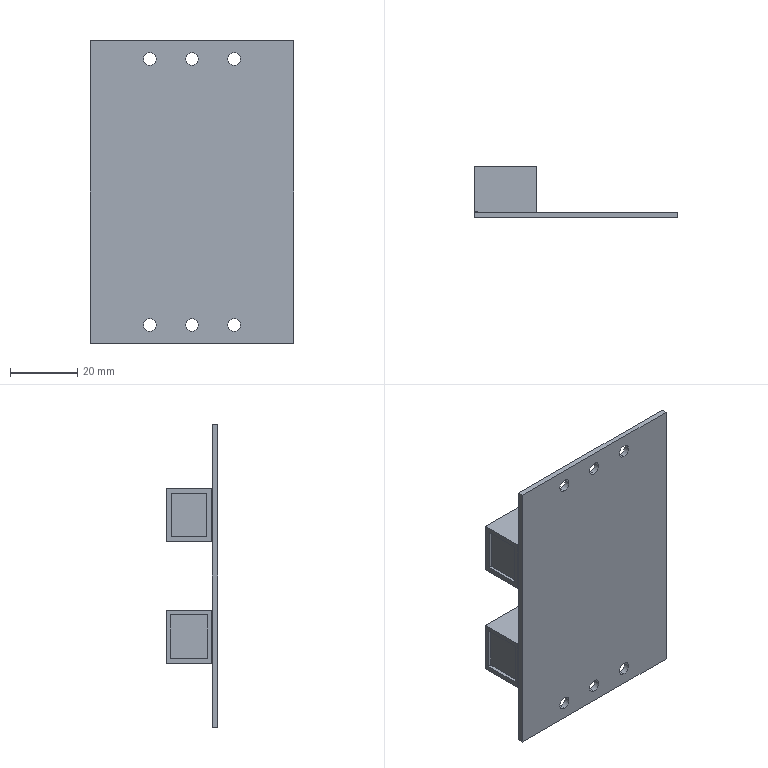Part | SolidWorks | features ICE 4, Extrusion 1 | 1 solid | 42 faces | box 60.4 x 15.3 x 89.7 mm | volume 16280 mm3 | plane 30 | cylinder 12 | commonest cylinder face diameters 3.8 x12
STEP:
#1=CARTESIAN_POINT('',(0.,0.,37.6));
#2=VERTEX_POINT('',#1);
#3=CARTESIAN_POINT('',(0.,0.,41.4));
#4=VERTEX_POINT('',#3);
#5=CARTESIAN_POINT('',(0.,0.,39.5));
#6=DIRECTION('',(0.,1.,0.));
#7=DIRECTION('',(0.,0.,1.));
#8=AXIS2_PLACEMENT_3D('',#5,#6,#7);
#9=CIRCLE('',#8,1.9);
#10=EDGE_CURVE('',#2,#4,#9,.T.);
#11=ORIENTED_EDGE('',*,*,#10,.F.);
#12=CARTESIAN_POINT('',(0.,1.6,37.6));
#13=VERTEX_POINT('',#12);
#14=CARTESIAN_POINT('',(0.,0.,37.6));
#15=DIRECTION('',(0.,1.,0.));
#16=VECTOR('',#15,1000.);
#17=LINE('',#14,#16);
#18=EDGE_CURVE('',#2,#13,#17,.T.);
#19=ORIENTED_EDGE('',*,*,#18,.T.);
#20=CARTESIAN_POINT('',(0.,1.6,41.4));
#21=VERTEX_POINT('',#20);
#22=CARTESIAN_POINT('',(0.,1.6,39.5));
#23=DIRECTION('',(0.,1.,0.));
#24=DIRECTION('',(0.,0.,1.));
#25=AXIS2_PLACEMENT_3D('',#22,#23,#24);
#26=CIRCLE('',#25,1.9);
#27=EDGE_CURVE('',#13,#21,#26,.T.);
#28=ORIENTED_EDGE('',*,*,#27,.T.);
#29=CARTESIAN_POINT('',(0.,0.,41.4));
#30=DIRECTION('',(0.,1.,0.));
#31=VECTOR('',#30,1000.);
#32=LINE('',#29,#31);
#33=EDGE_CURVE('',#4,#21,#32,.T.);
#34=ORIENTED_EDGE('',*,*,#33,.F.);
#35=EDGE_LOOP('',(#11,#19,#28,#34));
#36=FACE_OUTER_BOUND('',#35,.T.);
#37=CARTESIAN_POINT('',(0.,0.,39.5));
#38=DIRECTION('',(0.,1.,0.));
#39=DIRECTION('',(0.,0.,1.));
#40=AXIS2_PLACEMENT_3D('',#37,#38,#39);
#41=CYLINDRICAL_SURFACE('',#40,1.9);
#42=ADVANCED_FACE('',(#36),#41,.F.);
#43=CARTESIAN_POINT('',(0.,0.,-41.4));
#44=VERTEX_POINT('',#43);
#45=CARTESIAN_POINT('',(0.,0.,-37.6));
#46=VERTEX_POINT('',#45);
#47=CARTESIAN_POINT('',(0.,0.,-39.5));
#48=DIRECTION('',(0.,1.,0.));
#49=DIRECTION('',(0.,0.,1.));
#50=AXIS2_PLACEMENT_3D('',#47,#48,#49);
#51=CIRCLE('',#50,1.9);
#52=EDGE_CURVE('',#44,#46,#51,.T.);
#53=ORIENTED_EDGE('',*,*,#52,.F.);
#54=CARTESIAN_POINT('',(0.,1.6,-41.4));
#55=VERTEX_POINT('',#54);
#56=CARTESIAN_POINT('',(0.,0.,-41.4));
#57=DIRECTION('',(0.,1.,0.));
#58=VECTOR('',#57,1000.);
#59=LINE('',#56,#58);
#60=EDGE_CURVE('',#44,#55,#59,.T.);
#61=ORIENTED_EDGE('',*,*,#60,.T.);
#62=CARTESIAN_POINT('',(0.,1.6,-37.6));
#63=VERTEX_POINT('',#62);
#64=CARTESIAN_POINT('',(0.,1.6,-39.5));
#65=DIRECTION('',(0.,1.,0.));
#66=DIRECTION('',(0.,0.,1.));
#67=AXIS2_PLACEMENT_3D('',#64,#65,#66);
#68=CIRCLE('',#67,1.9);
#69=EDGE_CURVE('',#55,#63,#68,.T.);
#70=ORIENTED_EDGE('',*,*,#69,.T.);
#71=CARTESIAN_POINT('',(0.,0.,-37.6));
#72=DIRECTION('',(0.,1.,0.));
#73=VECTOR('',#72,1000.);
#74=LINE('',#71,#73);
#75=EDGE_CURVE('',#46,#63,#74,.T.);
#76=ORIENTED_EDGE('',*,*,#75,.F.);
#77=EDGE_LOOP('',(#53,#61,#70,#76));
#78=FACE_OUTER_BOUND('',#77,.T.);
#79=CARTESIAN_POINT('',(0.,0.,-39.5));
#80=DIRECTION('',(0.,1.,0.));
#81=DIRECTION('',(0.,0.,1.));
#82=AXIS2_PLACEMENT_3D('',#79,#80,#81);
#83=CYLINDRICAL_SURFACE('',#82,1.9);
#84=ADVANCED_FACE('',(#78),#83,.F.);
#85=CARTESIAN_POINT('',(12.5,0.,-41.4));
#86=VERTEX_POINT('',#85);
#87=CARTESIAN_POINT('',(12.5,0.,-37.6));
#88=VERTEX_POINT('',#87);
#89=CARTESIAN_POINT('',(12.5,0.,-39.5));
#90=DIRECTION('',(0.,1.,0.));
#91=DIRECTION('',(0.,0.,1.));
#92=AXIS2_PLACEMENT_3D('',#89,#90,#91);
#93=CIRCLE('',#92,1.9);
#94=EDGE_CURVE('',#86,#88,#93,.T.);
#95=ORIENTED_EDGE('',*,*,#94,.F.);
#96=CARTESIAN_POINT('',(12.5,1.6,-41.4));
#97=VERTEX_POINT('',#96);
#98=CARTESIAN_POINT('',(12.5,0.,-41.4));
#99=DIRECTION('',(0.,1.,0.));
#100=VECTOR('',#99,1000.);
#101=LINE('',#98,#100);
#102=EDGE_CURVE('',#86,#97,#101,.T.);
#103=ORIENTED_EDGE('',*,*,#102,.T.);
#104=CARTESIAN_POINT('',(12.5,1.6,-37.6));
#105=VERTEX_POINT('',#104);
#106=CARTESIAN_POINT('',(12.5,1.6,-39.5));
#107=DIRECTION('',(0.,1.,0.));
#108=DIRECTION('',(0.,0.,1.));
#109=AXIS2_PLACEMENT_3D('',#106,#107,#108);
#110=CIRCLE('',#109,1.9);
#111=EDGE_CURVE('',#97,#105,#110,.T.);
#112=ORIENTED_EDGE('',*,*,#111,.T.);
#113=CARTESIAN_POINT('',(12.5,0.,-37.6));
#114=DIRECTION('',(0.,1.,0.));
#115=VECTOR('',#114,1000.);
#116=LINE('',#113,#115);
#117=EDGE_CURVE('',#88,#105,#116,.T.);
#118=ORIENTED_EDGE('',*,*,#117,.F.);
#119=EDGE_LOOP('',(#95,#103,#112,#118));
#120=FACE_OUTER_BOUND('',#119,.T.);
#121=CARTESIAN_POINT('',(12.5,0.,-39.5));
#122=DIRECTION('',(0.,1.,0.));
#123=DIRECTION('',(0.,0.,1.));
#124=AXIS2_PLACEMENT_3D('',#121,#122,#123);
#125=CYLINDRICAL_SURFACE('',#124,1.9);
#126=ADVANCED_FACE('',(#120),#125,.F.);
#127=CARTESIAN_POINT('',(-12.5,0.,-41.4));
#128=VERTEX_POINT('',#127);
#129=CARTESIAN_POINT('',(-12.5,0.,-37.6));
#130=VERTEX_POINT('',#129);
#131=CARTESIAN_POINT('',(-12.5,0.,-39.5));
#132=DIRECTION('',(0.,1.,0.));
#133=DIRECTION('',(0.,0.,1.));
#134=AXIS2_PLACEMENT_3D('',#131,#132,#133);
#135=CIRCLE('',#134,1.9);
#136=EDGE_CURVE('',#128,#130,#135,.T.);
#137=ORIENTED_EDGE('',*,*,#136,.F.);
#138=CARTESIAN_POINT('',(-12.5,1.6,-41.4));
#139=VERTEX_POINT('',#138);
#140=CARTESIAN_POINT('',(-12.5,0.,-41.4));
#141=DIRECTION('',(0.,1.,0.));
#142=VECTOR('',#141,1000.);
#143=LINE('',#140,#142);
#144=EDGE_CURVE('',#128,#139,#143,.T.);
#145=ORIENTED_EDGE('',*,*,#144,.T.);
#146=CARTESIAN_POINT('',(-12.5,1.6,-37.6));
#147=VERTEX_POINT('',#146);
#148=CARTESIAN_POINT('',(-12.5,1.6,-39.5));
#149=DIRECTION('',(0.,1.,0.));
#150=DIRECTION('',(0.,0.,1.));
#151=AXIS2_PLACEMENT_3D('',#148,#149,#150);
#152=CIRCLE('',#151,1.9);
#153=EDGE_CURVE('',#139,#147,#152,.T.);
#154=ORIENTED_EDGE('',*,*,#153,.T.);
#155=CARTESIAN_POINT('',(-12.5,0.,-37.6));
#156=DIRECTION('',(0.,1.,0.));
#157=VECTOR('',#156,1000.);
#158=LINE('',#155,#157);
#159=EDGE_CURVE('',#130,#147,#158,.T.);
#160=ORIENTED_EDGE('',*,*,#159,.F.);
#161=EDGE_LOOP('',(#137,#145,#154,#160));
#162=FACE_OUTER_BOUND('',#161,.T.);
#163=CARTESIAN_POINT('',(-12.5,0.,-39.5));
#164=DIRECTION('',(0.,1.,0.));
#165=DIRECTION('',(0.,0.,1.));
#166=AXIS2_PLACEMENT_3D('',#163,#164,#165);
#167=CYLINDRICAL_SURFACE('',#166,1.9);
#168=ADVANCED_FACE('',(#162),#167,.F.);
#169=CARTESIAN_POINT('',(12.5,0.,37.6));
#170=VERTEX_POINT('',#169);
#171=CARTESIAN_POINT('',(12.5,0.,41.4));
#172=VERTEX_POINT('',#171);
#173=CARTESIAN_POINT('',(12.5,0.,39.5));
#174=DIRECTION('',(0.,1.,0.));
#175=DIRECTION('',(0.,0.,1.));
#176=AXIS2_PLACEMENT_3D('',#173,#174,#175);
#177=CIRCLE('',#176,1.9);
#178=EDGE_CURVE('',#170,#172,#177,.T.);
#179=ORIENTED_EDGE('',*,*,#178,.F.);
#180=CARTESIAN_POINT('',(12.5,1.6,37.6));
#181=VERTEX_POINT('',#180);
#182=CARTESIAN_POINT('',(12.5,0.,37.6));
#183=DIRECTION('',(0.,1.,0.));
#184=VECTOR('',#183,1000.);
#185=LINE('',#182,#184);
#186=EDGE_CURVE('',#170,#181,#185,.T.);
#187=ORIENTED_EDGE('',*,*,#186,.T.);
#188=CARTESIAN_POINT('',(12.5,1.6,41.4));
#189=VERTEX_POINT('',#188);
#190=CARTESIAN_POINT('',(12.5,1.6,39.5));
#191=DIRECTION('',(0.,1.,0.));
#192=DIRECTION('',(0.,0.,1.));
#193=AXIS2_PLACEMENT_3D('',#190,#191,#192);
#194=CIRCLE('',#193,1.9);
#195=EDGE_CURVE('',#181,#189,#194,.T.);
#196=ORIENTED_EDGE('',*,*,#195,.T.);
#197=CARTESIAN_POINT('',(12.5,0.,41.4));
#198=DIRECTION('',(0.,1.,0.));
#199=VECTOR('',#198,1000.);
#200=LINE('',#197,#199);
#201=EDGE_CURVE('',#172,#189,#200,.T.);
#202=ORIENTED_EDGE('',*,*,#201,.F.);
#203=EDGE_LOOP('',(#179,#187,#196,#202));
#204=FACE_OUTER_BOUND('',#203,.T.);
#205=CARTESIAN_POINT('',(12.5,0.,39.5));
#206=DIRECTION('',(0.,1.,0.));
#207=DIRECTION('',(0.,0.,1.));
#208=AXIS2_PLACEMENT_3D('',#205,#206,#207);
#209=CYLINDRICAL_SURFACE('',#208,1.9);
#210=ADVANCED_FACE('',(#204),#209,.F.);
#211=CARTESIAN_POINT('',(-12.5,0.,37.6));
#212=VERTEX_POINT('',#211);
#213=CARTESIAN_POINT('',(-12.5,0.,41.4));
#214=VERTEX_POINT('',#213);
#215=CARTESIAN_POINT('',(-12.5,0.,39.5));
#216=DIRECTION('',(0.,1.,0.));
#217=DIRECTION('',(0.,0.,1.));
#218=AXIS2_PLACEMENT_3D('',#215,#216,#217);
#219=CIRCLE('',#218,1.9);
#220=EDGE_CURVE('',#212,#214,#219,.T.);
#221=ORIENTED_EDGE('',*,*,#220,.F.);
#222=CARTESIAN_POINT('',(-12.5,1.6,37.6));
#223=VERTEX_POINT('',#222);
#224=CARTESIAN_POINT('',(-12.5,0.,37.6));
#225=DIRECTION('',(0.,1.,0.));
#226=VECTOR('',#225,1000.);
#227=LINE('',#224,#226);
#228=EDGE_CURVE('',#212,#223,#227,.T.);
#229=ORIENTED_EDGE('',*,*,#228,.T.);
#230=CARTESIAN_POINT('',(-12.5,1.6,41.4));
#231=VERTEX_POINT('',#230);
#232=CARTESIAN_POINT('',(-12.5,1.6,39.5));
#233=DIRECTION('',(0.,1.,0.));
#234=DIRECTION('',(0.,0.,1.));
#235=AXIS2_PLACEMENT_3D('',#232,#233,#234);
#236=CIRCLE('',#235,1.9);
#237=EDGE_CURVE('',#223,#231,#236,.T.);
#238=ORIENTED_EDGE('',*,*,#237,.T.);
#239=CARTESIAN_POINT('',(-12.5,0.,41.4));
#240=DIRECTION('',(0.,1.,0.));
#241=VECTOR('',#240,1000.);
#242=LINE('',#239,#241);
#243=EDGE_CURVE('',#214,#231,#242,.T.);
#244=ORIENTED_EDGE('',*,*,#243,.F.);
#245=EDGE_LOOP('',(#221,#229,#238,#244));
#246=FACE_OUTER_BOUND('',#245,.T.);
#247=CARTESIAN_POINT('',(-12.5,0.,39.5));
#248=DIRECTION('',(0.,1.,0.));
#249=DIRECTION('',(0.,0.,1.));
#250=AXIS2_PLACEMENT_3D('',#247,#248,#249);
#251=CYLINDRICAL_SURFACE('',#250,1.9);
#252=ADVANCED_FACE('',(#246),#251,.F.);
#253=CARTESIAN_POINT('',(-30.2,13.867,24.396));
#254=VERTEX_POINT('',#253);
#255=CARTESIAN_POINT('',(-30.2,13.867,11.604));
#256=VERTEX_POINT('',#255);
#257=CARTESIAN_POINT('',(-30.2,13.867,11.604));
#258=DIRECTION('',(0.,0.,-1.));
#259=VECTOR('',#258,1000.);
#260=LINE('',#257,#259);
#261=EDGE_CURVE('',#254,#256,#260,.T.);
#262=ORIENTED_EDGE('',*,*,#261,.F.);
#263=CARTESIAN_POINT('',(-30.2,3.233,24.396));
#264=VERTEX_POINT('',#263);
#265=CARTESIAN_POINT('',(-30.2,13.867,24.396));
#266=DIRECTION('',(0.,1.,0.));
#267=VECTOR('',#266,1000.);
#268=LINE('',#265,#267);
#269=EDGE_CURVE('',#264,#254,#268,.T.);
#270=ORIENTED_EDGE('',*,*,#269,.F.);
#271=CARTESIAN_POINT('',(-30.2,3.233,11.604));
#272=VERTEX_POINT('',#271);
#273=CARTESIAN_POINT('',(-30.2,3.233,11.604));
#274=DIRECTION('',(0.,0.,1.));
#275=VECTOR('',#274,1000.);
#276=LINE('',#273,#275);
#277=EDGE_CURVE('',#272,#264,#276,.T.);
#278=ORIENTED_EDGE('',*,*,#277,.F.);
#279=CARTESIAN_POINT('',(-30.2,13.867,11.604));
#280=DIRECTION('',(0.,-1.,0.));
#281=VECTOR('',#280,1000.);
#282=LINE('',#279,#281);
#283=EDGE_CURVE('',#256,#272,#282,.T.);
#284=ORIENTED_EDGE('',*,*,#283,.F.);
#285=EDGE_LOOP('',(#262,#270,#278,#284));
#286=FACE_BOUND('',#285,.T.);
#287=CARTESIAN_POINT('',(-30.2,15.3,10.1));
#288=VERTEX_POINT('',#287);
#289=CARTESIAN_POINT('',(-30.2,1.8,10.1));
#290=VERTEX_POINT('',#289);
#291=CARTESIAN_POINT('',(-30.2,15.3,10.1));
#292=DIRECTION('',(0.,-1.,0.));
#293=VECTOR('',#292,1000.);
#294=LINE('',#291,#293);
#295=EDGE_CURVE('',#288,#290,#294,.T.);
#296=ORIENTED_EDGE('',*,*,#295,.T.);
#297=CARTESIAN_POINT('',(-30.2,1.8,25.9));
#298=VERTEX_POINT('',#297);
#299=CARTESIAN_POINT('',(-30.2,1.8,-25.9));
#300=DIRECTION('',(0.,0.,-1.));
#301=VECTOR('',#300,1000.);
#302=LINE('',#299,#301);
#303=EDGE_CURVE('',#298,#290,#302,.T.);
#304=ORIENTED_EDGE('',*,*,#303,.F.);
#305=CARTESIAN_POINT('',(-30.2,15.3,25.9));
#306=VERTEX_POINT('',#305);
#307=CARTESIAN_POINT('',(-30.2,15.3,25.9));
#308=DIRECTION('',(0.,1.,0.));
#309=VECTOR('',#308,1000.);
#310=LINE('',#307,#309);
#311=EDGE_CURVE('',#298,#306,#310,.T.);
#312=ORIENTED_EDGE('',*,*,#311,.T.);
#313=CARTESIAN_POINT('',(-30.2,15.3,10.1));
#314=DIRECTION('',(0.,0.,-1.));
#315=VECTOR('',#314,1000.);
#316=LINE('',#313,#315);
#317=EDGE_CURVE('',#306,#288,#316,.T.);
#318=ORIENTED_EDGE('',*,*,#317,.T.);
#319=EDGE_LOOP('',(#296,#304,#312,#318));
#320=FACE_OUTER_BOUND('',#319,.T.);
#321=CARTESIAN_POINT('',(-30.2,1.6,-44.85));
#322=DIRECTION('',(1.,0.,0.));
#323=DIRECTION('',(0.,0.,-1.));
#324=AXIS2_PLACEMENT_3D('',#321,#322,#323);
#325=PLANE('',#324);
#326=ADVANCED_FACE('',(#286,#320),#325,.F.);
#327=CARTESIAN_POINT('',(-30.2,14.18,-11.503));
#328=VERTEX_POINT('',#327);
#329=CARTESIAN_POINT('',(-30.2,14.18,-24.497));
#330=VERTEX_POINT('',#329);
#331=CARTESIAN_POINT('',(-30.2,14.18,-24.497));
#332=DIRECTION('',(0.,0.,-1.));
#333=VECTOR('',#332,1000.);
#334=LINE('',#331,#333);
#335=EDGE_CURVE('',#328,#330,#334,.T.);
#336=ORIENTED_EDGE('',*,*,#335,.F.);
#337=CARTESIAN_POINT('',(-30.2,2.92,-11.503));
#338=VERTEX_POINT('',#337);
#339=CARTESIAN_POINT('',(-30.2,14.18,-11.503));
#340=DIRECTION('',(0.,1.,0.));
#341=VECTOR('',#340,1000.);
#342=LINE('',#339,#341);
#343=EDGE_CURVE('',#338,#328,#342,.T.);
#344=ORIENTED_EDGE('',*,*,#343,.F.);
#345=CARTESIAN_POINT('',(-30.2,2.92,-24.497));
#346=VERTEX_POINT('',#345);
#347=CARTESIAN_POINT('',(-30.2,2.92,-24.497));
#348=DIRECTION('',(0.,0.,1.));
#349=VECTOR('',#348,1000.);
#350=LINE('',#347,#349);
#351=EDGE_CURVE('',#346,#338,#350,.T.);
#352=ORIENTED_EDGE('',*,*,#351,.F.);
#353=CARTESIAN_POINT('',(-30.2,14.18,-24.497));
#354=DIRECTION('',(0.,-1.,0.));
#355=VECTOR('',#354,1000.);
#356=LINE('',#353,#355);
#357=EDGE_CURVE('',#330,#346,#356,.T.);
#358=ORIENTED_EDGE('',*,*,#357,.F.);
#359=EDGE_LOOP('',(#336,#344,#352,#358));
#360=FACE_BOUND('',#359,.T.);
#361=CARTESIAN_POINT('',(-30.2,15.3,-25.9));
#362=VERTEX_POINT('',#361);
#363=CARTESIAN_POINT('',(-30.2,1.8,-25.9));
#364=VERTEX_POINT('',#363);
#365=CARTESIAN_POINT('',(-30.2,15.3,-25.9));
#366=DIRECTION('',(0.,-1.,0.));
#367=VECTOR('',#366,1000.);
#368=LINE('',#365,#367);
#369=EDGE_CURVE('',#362,#364,#368,.T.);
#370=ORIENTED_EDGE('',*,*,#369,.T.);
#371=CARTESIAN_POINT('',(-30.2,1.8,-10.1));
#372=VERTEX_POINT('',#371);
#373=CARTESIAN_POINT('',(-30.2,1.8,-25.9));
#374=DIRECTION('',(0.,0.,-1.));
#375=VECTOR('',#374,1000.);
#376=LINE('',#373,#375);
#377=EDGE_CURVE('',#372,#364,#376,.T.);
#378=ORIENTED_EDGE('',*,*,#377,.F.);
#379=CARTESIAN_POINT('',(-30.2,15.3,-10.1));
#380=VERTEX_POINT('',#379);
#381=CARTESIAN_POINT('',(-30.2,15.3,-10.1));
#382=DIRECTION('',(0.,1.,0.));
#383=VECTOR('',#382,1000.);
#384=LINE('',#381,#383);
#385=EDGE_CURVE('',#372,#380,#384,.T.);
#386=ORIENTED_EDGE('',*,*,#385,.T.);
#387=CARTESIAN_POINT('',(-30.2,15.3,-25.9));
#388=DIRECTION('',(0.,0.,-1.));
#389=VECTOR('',#388,1000.);
#390=LINE('',#387,#389);
#391=EDGE_CURVE('',#380,#362,#390,.T.);
#392=ORIENTED_EDGE('',*,*,#391,.T.);
#393=EDGE_LOOP('',(#370,#378,#386,#392));
#394=FACE_OUTER_BOUND('',#393,.T.);
#395=CARTESIAN_POINT('',(-30.2,1.6,-44.85));
#396=DIRECTION('',(1.,0.,0.));
#397=DIRECTION('',(0.,0.,-1.));
#398=AXIS2_PLACEMENT_3D('',#395,#396,#397);
#399=PLANE('',#398);
#400=ADVANCED_FACE('',(#360,#394),#399,.F.);
#401=CARTESIAN_POINT('',(30.2,0.,44.85));
#402=VERTEX_POINT('',#401);
#403=CARTESIAN_POINT('',(30.2,0.,-44.85));
#404=VERTEX_POINT('',#403);
#405=CARTESIAN_POINT('',(30.2,0.,-44.85));
#406=DIRECTION('',(0.,0.,-1.));
#407=VECTOR('',#406,1000.);
#408=LINE('',#405,#407);
#409=EDGE_CURVE('',#402,#404,#408,.T.);
#410=ORIENTED_EDGE('',*,*,#409,.T.);
#411=CARTESIAN_POINT('',(30.2,1.6,-44.85));
#412=VERTEX_POINT('',#411);
#413=CARTESIAN_POINT('',(30.2,1.6,-44.85));
#414=DIRECTION('',(0.,-1.,0.));
#415=VECTOR('',#414,1000.);
#416=LINE('',#413,#415);
#417=EDGE_CURVE('',#412,#404,#416,.T.);
#418=ORIENTED_EDGE('',*,*,#417,.F.);
#419=CARTESIAN_POINT('',(30.2,1.6,44.85));
#420=VERTEX_POINT('',#419);
#421=CARTESIAN_POINT('',(30.2,1.6,-44.85));
#422=DIRECTION('',(0.,0.,-1.));
#423=VECTOR('',#422,1000.);
#424=LINE('',#421,#423);
#425=EDGE_CURVE('',#420,#412,#424,.T.);
#426=ORIENTED_EDGE('',*,*,#425,.F.);
#427=CARTESIAN_POINT('',(30.2,1.6,44.85));
#428=DIRECTION('',(0.,-1.,0.));
#429=VECTOR('',#428,1000.);
#430=LINE('',#427,#429);
#431=EDGE_CURVE('',#420,#402,#430,.T.);
#432=ORIENTED_EDGE('',*,*,#431,.T.);
#433=EDGE_LOOP('',(#410,#418,#426,#432));
#434=FACE_OUTER_BOUND('',#433,.T.);
#435=CARTESIAN_POINT('',(30.2,1.6,-44.85));
#436=DIRECTION('',(-1.,0.,0.));
#437=DIRECTION('',(0.,0.,1.));
#438=AXIS2_PLACEMENT_3D('',#435,#436,#437);
#439=PLANE('',#438);
#440=ADVANCED_FACE('',(#434),#439,.F.);
#441=CARTESIAN_POINT('',(-30.2,0.,-44.85));
#442=VERTEX_POINT('',#441);
#443=CARTESIAN_POINT('',(-30.2,0.,-44.85));
#444=DIRECTION('',(-1.,0.,0.));
#445=VECTOR('',#444,1000.);
#446=LINE('',#443,#445);
#447=EDGE_CURVE('',#404,#442,#446,.T.);
#448=ORIENTED_EDGE('',*,*,#447,.T.);
#449=CARTESIAN_POINT('',(-30.2,1.6,-44.85));
#450=VERTEX_POINT('',#449);
#451=CARTESIAN_POINT('',(-30.2,1.6,-44.85));
#452=DIRECTION('',(0.,-1.,0.));
#453=VECTOR('',#452,1000.);
#454=LINE('',#451,#453);
#455=EDGE_CURVE('',#450,#442,#454,.T.);
#456=ORIENTED_EDGE('',*,*,#455,.F.);
#457=CARTESIAN_POINT('',(-30.2,1.6,-44.85));
#458=DIRECTION('',(-1.,0.,0.));
#459=VECTOR('',#458,1000.);
#460=LINE('',#457,#459);
#461=EDGE_CURVE('',#412,#450,#460,.T.);
#462=ORIENTED_EDGE('',*,*,#461,.F.);
#463=ORIENTED_EDGE('',*,*,#417,.T.);
#464=EDGE_LOOP('',(#448,#456,#462,#463));
#465=FACE_OUTER_BOUND('',#464,.T.);
#466=CARTESIAN_POINT('',(-30.2,1.6,-44.85));
#467=DIRECTION('',(0.,0.,1.));
#468=DIRECTION('',(1.,0.,0.));
#469=AXIS2_PLACEMENT_3D('',#466,#467,#468);
#470=PLANE('',#469);
#471=ADVANCED_FACE('',(#465),#470,.F.);
#472=CARTESIAN_POINT('',(-30.2,1.6,44.85));
#473=VERTEX_POINT('',#472);
#474=CARTESIAN_POINT('',(-30.2,0.,44.85));
#475=VERTEX_POINT('',#474);
#476=CARTESIAN_POINT('',(-30.2,1.6,44.85));
#477=DIRECTION('',(0.,-1.,0.));
#478=VECTOR('',#477,1000.);
#479=LINE('',#476,#478);
#480=EDGE_CURVE('',#473,#475,#479,.T.);
#481=ORIENTED_EDGE('',*,*,#480,.F.);
#482=CARTESIAN_POINT('',(-30.2,1.6,-44.85));
#483=DIRECTION('',(0.,0.,1.));
#484=VECTOR('',#483,1000.);
#485=LINE('',#482,#484);
#486=EDGE_CURVE('',#450,#473,#485,.T.);
#487=ORIENTED_EDGE('',*,*,#486,.F.);
#488=ORIENTED_EDGE('',*,*,#455,.T.);
#489=CARTESIAN_POINT('',(-30.2,0.,-44.85));
#490=DIRECTION('',(0.,0.,1.));
#491=VECTOR('',#490,1000.);
#492=LINE('',#489,#491);
#493=EDGE_CURVE('',#442,#475,#492,.T.);
#494=ORIENTED_EDGE('',*,*,#493,.T.);
#495=EDGE_LOOP('',(#481,#487,#488,#494));
#496=FACE_OUTER_BOUND('',#495,.T.);
#497=CARTESIAN_POINT('',(-30.2,1.6,-44.85));
#498=DIRECTION('',(1.,0.,0.));
#499=DIRECTION('',(0.,0.,-1.));
#500=AXIS2_PLACEMENT_3D('',#497,#498,#499);
#501=PLANE('',#500);
#502=ADVANCED_FACE('',(#496),#501,.F.);
#503=CARTESIAN_POINT('',(-30.2,0.,44.85));
#504=DIRECTION('',(1.,0.,0.));
#505=VECTOR('',#504,1000.);
#506=LINE('',#503,#505);
#507=EDGE_CURVE('',#475,#402,#506,.T.);
#508=ORIENTED_EDGE('',*,*,#507,.T.);
#509=ORIENTED_EDGE('',*,*,#431,.F.);
#510=CARTESIAN_POINT('',(-30.2,1.6,44.85));
#511=DIRECTION('',(1.,0.,0.));
#512=VECTOR('',#511,1000.);
#513=LINE('',#510,#512);
#514=EDGE_CURVE('',#473,#420,#513,.T.);
#515=ORIENTED_EDGE('',*,*,#514,.F.);
#516=ORIENTED_EDGE('',*,*,#480,.T.);
#517=EDGE_LOOP('',(#508,#509,#515,#516));
#518=FACE_OUTER_BOUND('',#517,.T.);
#519=CARTESIAN_POINT('',(-30.2,1.6,44.85));
#520=DIRECTION('',(0.,0.,-1.));
#521=DIRECTION('',(-1.,0.,0.));
#522=AXIS2_PLACEMENT_3D('',#519,#520,#521);
#523=PLANE('',#522);
#524=ADVANCED_FACE('',(#518),#523,.F.);
#525=CARTESIAN_POINT('',(-11.7,1.6,-10.1));
#526=VERTEX_POINT('',#525);
#527=CARTESIAN_POINT('',(-29.2,1.6,-10.1));
#528=VERTEX_POINT('',#527);
#529=CARTESIAN_POINT('',(-11.7,1.6,-10.1));
#530=DIRECTION('',(-1.,0.,0.));
#531=VECTOR('',#530,1000.);
#532=LINE('',#529,#531);
#533=EDGE_CURVE('',#526,#528,#532,.T.);
#534=ORIENTED_EDGE('',*,*,#533,.T.);
#535=CARTESIAN_POINT('',(-29.2,1.6,-25.9));
#536=VERTEX_POINT('',#535);
#537=CARTESIAN_POINT('',(-29.2,1.6,-25.9));
#538=DIRECTION('',(0.,0.,1.));
#539=VECTOR('',#538,1000.);
#540=LINE('',#537,#539);
#541=EDGE_CURVE('',#536,#528,#540,.T.);
#542=ORIENTED_EDGE('',*,*,#541,.F.);
#543=CARTESIAN_POINT('',(-11.7,1.6,-25.9));
#544=VERTEX_POINT('',#543);
#545=CARTESIAN_POINT('',(-11.7,1.6,-25.9));
#546=DIRECTION('',(-1.,0.,0.));
#547=VECTOR('',#546,1000.);
#548=LINE('',#545,#547);
#549=EDGE_CURVE('',#544,#536,#548,.T.);
#550=ORIENTED_EDGE('',*,*,#549,.F.);
#551=CARTESIAN_POINT('',(-11.7,1.6,-25.9));
#552=DIRECTION('',(0.,0.,1.));
#553=VECTOR('',#552,1000.);
#554=LINE('',#551,#553);
#555=EDGE_CURVE('',#544,#526,#554,.T.);
#556=ORIENTED_EDGE('',*,*,#555,.T.);
#557=EDGE_LOOP('',(#534,#542,#550,#556));
#558=FACE_BOUND('',#557,.T.);
#559=ORIENTED_EDGE('',*,*,#486,.T.);
#560=ORIENTED_EDGE('',*,*,#514,.T.);
#561=ORIENTED_EDGE('',*,*,#425,.T.);
#562=ORIENTED_EDGE('',*,*,#461,.T.);
#563=EDGE_LOOP('',(#559,#560,#561,#562));
#564=FACE_OUTER_BOUND('',#563,.T.);
#565=CARTESIAN_POINT('',(-29.2,1.6,10.1));
#566=VERTEX_POINT('',#565);
#567=CARTESIAN_POINT('',(-29.2,1.6,25.9));
#568=VERTEX_POINT('',#567);
#569=CARTESIAN_POINT('',(-29.2,1.6,-25.9));
#570=DIRECTION('',(0.,0.,1.));
#571=VECTOR('',#570,1000.);
#572=LINE('',#569,#571);
#573=EDGE_CURVE('',#566,#568,#572,.T.);
#574=ORIENTED_EDGE('',*,*,#573,.F.);
#575=CARTESIAN_POINT('',(-11.7,1.6,10.1));
#576=VERTEX_POINT('',#575);
#577=CARTESIAN_POINT('',(-11.7,1.6,10.1));
#578=DIRECTION('',(-1.,0.,0.));
#579=VECTOR('',#578,1000.);
#580=LINE('',#577,#579);
#581=EDGE_CURVE('',#576,#566,#580,.T.);
#582=ORIENTED_EDGE('',*,*,#581,.F.);
#583=CARTESIAN_POINT('',(-11.7,1.6,25.9));
#584=VERTEX_POINT('',#583);
#585=CARTESIAN_POINT('',(-11.7,1.6,10.1));
#586=DIRECTION('',(0.,0.,1.));
#587=VECTOR('',#586,1000.);
#588=LINE('',#585,#587);
#589=EDGE_CURVE('',#576,#584,#588,.T.);
#590=ORIENTED_EDGE('',*,*,#589,.T.);
#591=CARTESIAN_POINT('',(-11.7,1.6,25.9));
#592=DIRECTION('',(-1.,0.,0.));
#593=VECTOR('',#592,1000.);
#594=LINE('',#591,#593);
#595=EDGE_CURVE('',#584,#568,#594,.T.);
#596=ORIENTED_EDGE('',*,*,#595,.T.);
#597=EDGE_LOOP('',(#574,#582,#590,#596));
#598=FACE_BOUND('',#597,.T.);
#599=CARTESIAN_POINT('',(0.,1.6,39.5));
#600=DIRECTION('',(0.,1.,0.));
#601=DIRECTION('',(0.,0.,1.));
#602=AXIS2_PLACEMENT_3D('',#599,#600,#601);
#603=CIRCLE('',#602,1.9);
#604=EDGE_CURVE('',#21,#13,#603,.T.);
#605=ORIENTED_EDGE('',*,*,#604,.F.);
#606=ORIENTED_EDGE('',*,*,#27,.F.);
#607=EDGE_LOOP('',(#605,#606));
#608=FACE_BOUND('',#607,.T.);
#609=CARTESIAN_POINT('',(0.,1.6,-39.5));
#610=DIRECTION('',(0.,1.,0.));
#611=DIRECTION('',(0.,0.,1.));
#612=AXIS2_PLACEMENT_3D('',#609,#610,#611);
#613=CIRCLE('',#612,1.9);
#614=EDGE_CURVE('',#63,#55,#613,.T.);
#615=ORIENTED_EDGE('',*,*,#614,.F.);
#616=ORIENTED_EDGE('',*,*,#69,.F.);
#617=EDGE_LOOP('',(#615,#616));
#618=FACE_BOUND('',#617,.T.);
#619=CARTESIAN_POINT('',(12.5,1.6,-39.5));
#620=DIRECTION('',(0.,1.,0.));
#621=DIRECTION('',(0.,0.,1.));
#622=AXIS2_PLACEMENT_3D('',#619,#620,#621);
#623=CIRCLE('',#622,1.9);
#624=EDGE_CURVE('',#105,#97,#623,.T.);
#625=ORIENTED_EDGE('',*,*,#624,.F.);
#626=ORIENTED_EDGE('',*,*,#111,.F.);
#627=EDGE_LOOP('',(#625,#626));
#628=FACE_BOUND('',#627,.T.);
#629=CARTESIAN_POINT('',(-12.5,1.6,-39.5));
#630=DIRECTION('',(0.,1.,0.));
#631=DIRECTION('',(0.,0.,1.));
#632=AXIS2_PLACEMENT_3D('',#629,#630,#631);
#633=CIRCLE('',#632,1.9);
#634=EDGE_CURVE('',#147,#139,#633,.T.);
#635=ORIENTED_EDGE('',*,*,#634,.F.);
#636=ORIENTED_EDGE('',*,*,#153,.F.);
#637=EDGE_LOOP('',(#635,#636));
#638=FACE_BOUND('',#637,.T.);
#639=CARTESIAN_POINT('',(12.5,1.6,39.5));
#640=DIRECTION('',(0.,1.,0.));
#641=DIRECTION('',(0.,0.,1.));
#642=AXIS2_PLACEMENT_3D('',#639,#640,#641);
#643=CIRCLE('',#642,1.9);
#644=EDGE_CURVE('',#189,#181,#643,.T.);
#645=ORIENTED_EDGE('',*,*,#644,.F.);
#646=ORIENTED_EDGE('',*,*,#195,.F.);
#647=EDGE_LOOP('',(#645,#646));
#648=FACE_BOUND('',#647,.T.);
#649=CARTESIAN_POINT('',(-12.5,1.6,39.5));
#650=DIRECTION('',(0.,1.,0.));
#651=DIRECTION('',(0.,0.,1.));
#652=AXIS2_PLACEMENT_3D('',#649,#650,#651);
#653=CIRCLE('',#652,1.9);
#654=EDGE_CURVE('',#231,#223,#653,.T.);
#655=ORIENTED_EDGE('',*,*,#654,.F.);
#656=ORIENTED_EDGE('',*,*,#237,.F.);
#657=EDGE_LOOP('',(#655,#656));
#658=FACE_BOUND('',#657,.T.);
#659=CARTESIAN_POINT('',(0.,1.6,0.));
#660=DIRECTION('',(0.,1.,0.));
#661=DIRECTION('',(0.,0.,1.));
#662=AXIS2_PLACEMENT_3D('',#659,#660,#661);
#663=PLANE('',#662);
#664=ADVANCED_FACE('',(#558,#564,#598,#608,#618,#628,#638,#648,#658),#663,.T.);
#665=CARTESIAN_POINT('',(0.,0.,39.5));
#666=DIRECTION('',(0.,1.,0.));
#667=DIRECTION('',(0.,0.,1.));
#668=AXIS2_PLACEMENT_3D('',#665,#666,#667);
#669=CIRCLE('',#668,1.9);
#670=EDGE_CURVE('',#4,#2,#669,.T.);
#671=ORIENTED_EDGE('',*,*,#670,.T.);
#672=ORIENTED_EDGE('',*,*,#10,.T.);
#673=EDGE_LOOP('',(#671,#672));
#674=FACE_BOUND('',#673,.T.);
#675=CARTESIAN_POINT('',(0.,0.,-39.5));
#676=DIRECTION('',(0.,1.,0.));
#677=DIRECTION('',(0.,0.,1.));
#678=AXIS2_PLACEMENT_3D('',#675,#676,#677);
#679=CIRCLE('',#678,1.9);
#680=EDGE_CURVE('',#46,#44,#679,.T.);
#681=ORIENTED_EDGE('',*,*,#680,.T.);
#682=ORIENTED_EDGE('',*,*,#52,.T.);
#683=EDGE_LOOP('',(#681,#682));
#684=FACE_BOUND('',#683,.T.);
#685=CARTESIAN_POINT('',(12.5,0.,-39.5));
#686=DIRECTION('',(0.,1.,0.));
#687=DIRECTION('',(0.,0.,1.));
#688=AXIS2_PLACEMENT_3D('',#685,#686,#687);
#689=CIRCLE('',#688,1.9);
#690=EDGE_CURVE('',#88,#86,#689,.T.);
#691=ORIENTED_EDGE('',*,*,#690,.T.);
#692=ORIENTED_EDGE('',*,*,#94,.T.);
#693=EDGE_LOOP('',(#691,#692));
#694=FACE_BOUND('',#693,.T.);
#695=CARTESIAN_POINT('',(-12.5,0.,-39.5));
#696=DIRECTION('',(0.,1.,0.));
#697=DIRECTION('',(0.,0.,1.));
#698=AXIS2_PLACEMENT_3D('',#695,#696,#697);
#699=CIRCLE('',#698,1.9);
#700=EDGE_CURVE('',#130,#128,#699,.T.);
#701=ORIENTED_EDGE('',*,*,#700,.T.);
#702=ORIENTED_EDGE('',*,*,#136,.T.);
#703=EDGE_LOOP('',(#701,#702));
#704=FACE_BOUND('',#703,.T.);
#705=CARTESIAN_POINT('',(12.5,0.,39.5));
#706=DIRECTION('',(0.,1.,0.));
#707=DIRECTION('',(0.,0.,1.));
#708=AXIS2_PLACEMENT_3D('',#705,#706,#707);
#709=CIRCLE('',#708,1.9);
#710=EDGE_CURVE('',#172,#170,#709,.T.);
#711=ORIENTED_EDGE('',*,*,#710,.T.);
#712=ORIENTED_EDGE('',*,*,#178,.T.);
#713=EDGE_LOOP('',(#711,#712));
#714=FACE_BOUND('',#713,.T.);
#715=CARTESIAN_POINT('',(-12.5,0.,39.5));
#716=DIRECTION('',(0.,1.,0.));
#717=DIRECTION('',(0.,0.,1.));
#718=AXIS2_PLACEMENT_3D('',#715,#716,#717);
#719=CIRCLE('',#718,1.9);
#720=EDGE_CURVE('',#214,#212,#719,.T.);
#721=ORIENTED_EDGE('',*,*,#720,.T.);
#722=ORIENTED_EDGE('',*,*,#220,.T.);
#723=EDGE_LOOP('',(#721,#722));
#724=FACE_BOUND('',#723,.T.);
#725=ORIENTED_EDGE('',*,*,#409,.F.);
#726=ORIENTED_EDGE('',*,*,#507,.F.);
#727=ORIENTED_EDGE('',*,*,#493,.F.);
#728=ORIENTED_EDGE('',*,*,#447,.F.);
#729=EDGE_LOOP('',(#725,#726,#727,#728));
#730=FACE_OUTER_BOUND('',#729,.T.);
#731=CARTESIAN_POINT('',(0.,0.,0.));
#732=DIRECTION('',(0.,1.,0.));
#733=DIRECTION('',(0.,0.,1.));
#734=AXIS2_PLACEMENT_3D('',#731,#732,#733);
#735=PLANE('',#734);
#736=ADVANCED_FACE('',(#674,#684,#694,#704,#714,#724,#730),#735,.F.);
#737=ORIENTED_EDGE('',*,*,#228,.F.);
#738=ORIENTED_EDGE('',*,*,#720,.F.);
#739=ORIENTED_EDGE('',*,*,#243,.T.);
#740=ORIENTED_EDGE('',*,*,#654,.T.);
#741=EDGE_LOOP('',(#737,#738,#739,#740));
#742=FACE_OUTER_BOUND('',#741,.T.);
#743=CARTESIAN_POINT('',(-12.5,0.,39.5));
#744=DIRECTION('',(0.,1.,0.));
#745=DIRECTION('',(0.,0.,1.));
#746=AXIS2_PLACEMENT_3D('',#743,#744,#745);
#747=CYLINDRICAL_SURFACE('',#746,1.9);
#748=ADVANCED_FACE('',(#742),#747,.F.);
#749=ORIENTED_EDGE('',*,*,#186,.F.);
#750=ORIENTED_EDGE('',*,*,#710,.F.);
#751=ORIENTED_EDGE('',*,*,#201,.T.);
#752=ORIENTED_EDGE('',*,*,#644,.T.);
#753=EDGE_LOOP('',(#749,#750,#751,#752));
#754=FACE_OUTER_BOUND('',#753,.T.);
#755=CARTESIAN_POINT('',(12.5,0.,39.5));
#756=DIRECTION('',(0.,1.,0.));
#757=DIRECTION('',(0.,0.,1.));
#758=AXIS2_PLACEMENT_3D('',#755,#756,#757);
#759=CYLINDRICAL_SURFACE('',#758,1.9);
#760=ADVANCED_FACE('',(#754),#759,.F.);
#761=ORIENTED_EDGE('',*,*,#144,.F.);
#762=ORIENTED_EDGE('',*,*,#700,.F.);
#763=ORIENTED_EDGE('',*,*,#159,.T.);
#764=ORIENTED_EDGE('',*,*,#634,.T.);
#765=EDGE_LOOP('',(#761,#762,#763,#764));
#766=FACE_OUTER_BOUND('',#765,.T.);
#767=CARTESIAN_POINT('',(-12.5,0.,-39.5));
#768=DIRECTION('',(0.,1.,0.));
#769=DIRECTION('',(0.,0.,1.));
#770=AXIS2_PLACEMENT_3D('',#767,#768,#769);
#771=CYLINDRICAL_SURFACE('',#770,1.9);
#772=ADVANCED_FACE('',(#766),#771,.F.);
#773=ORIENTED_EDGE('',*,*,#102,.F.);
#774=ORIENTED_EDGE('',*,*,#690,.F.);
#775=ORIENTED_EDGE('',*,*,#117,.T.);
#776=ORIENTED_EDGE('',*,*,#624,.T.);
#777=EDGE_LOOP('',(#773,#774,#775,#776));
#778=FACE_OUTER_BOUND('',#777,.T.);
#779=CARTESIAN_POINT('',(12.5,0.,-39.5));
#780=DIRECTION('',(0.,1.,0.));
#781=DIRECTION('',(0.,0.,1.));
#782=AXIS2_PLACEMENT_3D('',#779,#780,#781);
#783=CYLINDRICAL_SURFACE('',#782,1.9);
#784=ADVANCED_FACE('',(#778),#783,.F.);
#785=ORIENTED_EDGE('',*,*,#60,.F.);
#786=ORIENTED_EDGE('',*,*,#680,.F.);
#787=ORIENTED_EDGE('',*,*,#75,.T.);
#788=ORIENTED_EDGE('',*,*,#614,.T.);
#789=EDGE_LOOP('',(#785,#786,#787,#788));
#790=FACE_OUTER_BOUND('',#789,.T.);
#791=CARTESIAN_POINT('',(0.,0.,-39.5));
#792=DIRECTION('',(0.,1.,0.));
#793=DIRECTION('',(0.,0.,1.));
#794=AXIS2_PLACEMENT_3D('',#791,#792,#793);
#795=CYLINDRICAL_SURFACE('',#794,1.9);
#796=ADVANCED_FACE('',(#790),#795,.F.);
#797=ORIENTED_EDGE('',*,*,#18,.F.);
#798=ORIENTED_EDGE('',*,*,#670,.F.);
#799=ORIENTED_EDGE('',*,*,#33,.T.);
#800=ORIENTED_EDGE('',*,*,#604,.T.);
#801=EDGE_LOOP('',(#797,#798,#799,#800));
#802=FACE_OUTER_BOUND('',#801,.T.);
#803=CARTESIAN_POINT('',(0.,0.,39.5));
#804=DIRECTION('',(0.,1.,0.));
#805=DIRECTION('',(0.,0.,1.));
#806=AXIS2_PLACEMENT_3D('',#803,#804,#805);
#807=CYLINDRICAL_SURFACE('',#806,1.9);
#808=ADVANCED_FACE('',(#802),#807,.F.);
#809=CARTESIAN_POINT('',(-29.2,1.8,10.1));
#810=VERTEX_POINT('',#809);
#811=CARTESIAN_POINT('',(-11.7,1.8,10.1));
#812=DIRECTION('',(1.,0.,0.));
#813=VECTOR('',#812,1000.);
#814=LINE('',#811,#813);
#815=EDGE_CURVE('',#290,#810,#814,.T.);
#816=ORIENTED_EDGE('',*,*,#815,.F.);
#817=ORIENTED_EDGE('',*,*,#295,.F.);
#818=CARTESIAN_POINT('',(-11.7,15.3,10.1));
#819=VERTEX_POINT('',#818);
#820=CARTESIAN_POINT('',(-11.7,15.3,10.1));
#821=DIRECTION('',(-1.,0.,0.));
#822=VECTOR('',#821,1000.);
#823=LINE('',#820,#822);
#824=EDGE_CURVE('',#819,#288,#823,.T.);
#825=ORIENTED_EDGE('',*,*,#824,.F.);
#826=CARTESIAN_POINT('',(-11.7,15.3,10.1));
#827=DIRECTION('',(0.,-1.,0.));
#828=VECTOR('',#827,1000.);
#829=LINE('',#826,#828);
#830=EDGE_CURVE('',#819,#576,#829,.T.);
#831=ORIENTED_EDGE('',*,*,#830,.T.);
#832=ORIENTED_EDGE('',*,*,#581,.T.);
#833=CARTESIAN_POINT('',(-29.2,15.3,10.1));
#834=DIRECTION('',(0.,-1.,0.));
#835=VECTOR('',#834,1000.);
#836=LINE('',#833,#835);
#837=EDGE_CURVE('',#810,#566,#836,.T.);
#838=ORIENTED_EDGE('',*,*,#837,.F.);
#839=EDGE_LOOP('',(#816,#817,#825,#831,#832,#838));
#840=FACE_OUTER_BOUND('',#839,.T.);
#841=CARTESIAN_POINT('',(-11.7,15.3,10.1));
#842=DIRECTION('',(0.,0.,-1.));
#843=DIRECTION('',(0.,1.,0.));
#844=AXIS2_PLACEMENT_3D('',#841,#842,#843);
#845=PLANE('',#844);
#846=ADVANCED_FACE('',(#840),#845,.T.);
#847=ORIENTED_EDGE('',*,*,#317,.F.);
#848=CARTESIAN_POINT('',(-11.7,15.3,25.9));
#849=VERTEX_POINT('',#848);
#850=CARTESIAN_POINT('',(-11.7,15.3,25.9));
#851=DIRECTION('',(-1.,0.,0.));
#852=VECTOR('',#851,1000.);
#853=LINE('',#850,#852);
#854=EDGE_CURVE('',#849,#306,#853,.T.);
#855=ORIENTED_EDGE('',*,*,#854,.F.);
#856=CARTESIAN_POINT('',(-11.7,15.3,10.1));
#857=DIRECTION('',(0.,0.,-1.));
#858=VECTOR('',#857,1000.);
#859=LINE('',#856,#858);
#860=EDGE_CURVE('',#849,#819,#859,.T.);
#861=ORIENTED_EDGE('',*,*,#860,.T.);
#862=ORIENTED_EDGE('',*,*,#824,.T.);
#863=EDGE_LOOP('',(#847,#855,#861,#862));
#864=FACE_OUTER_BOUND('',#863,.T.);
#865=CARTESIAN_POINT('',(-11.7,15.3,10.1));
#866=DIRECTION('',(0.,1.,0.));
#867=DIRECTION('',(0.,0.,1.));
#868=AXIS2_PLACEMENT_3D('',#865,#866,#867);
#869=PLANE('',#868);
#870=ADVANCED_FACE('',(#864),#869,.T.);
#871=CARTESIAN_POINT('',(-29.2,1.8,25.9));
#872=VERTEX_POINT('',#871);
#873=CARTESIAN_POINT('',(-29.2,1.8,25.9));
#874=DIRECTION('',(-1.,0.,0.));
#875=VECTOR('',#874,1000.);
#876=LINE('',#873,#875);
#877=EDGE_CURVE('',#872,#298,#876,.T.);
#878=ORIENTED_EDGE('',*,*,#877,.F.);
#879=CARTESIAN_POINT('',(-29.2,1.6,25.9));
#880=DIRECTION('',(0.,1.,0.));
#881=VECTOR('',#880,1000.);
#882=LINE('',#879,#881);
#883=EDGE_CURVE('',#568,#872,#882,.T.);
#884=ORIENTED_EDGE('',*,*,#883,.F.);
#885=ORIENTED_EDGE('',*,*,#595,.F.);
#886=CARTESIAN_POINT('',(-11.7,15.3,25.9));
#887=DIRECTION('',(0.,1.,0.));
#888=VECTOR('',#887,1000.);
#889=LINE('',#886,#888);
#890=EDGE_CURVE('',#584,#849,#889,.T.);
#891=ORIENTED_EDGE('',*,*,#890,.T.);
#892=ORIENTED_EDGE('',*,*,#854,.T.);
#893=ORIENTED_EDGE('',*,*,#311,.F.);
#894=EDGE_LOOP('',(#878,#884,#885,#891,#892,#893));
#895=FACE_OUTER_BOUND('',#894,.T.);
#896=CARTESIAN_POINT('',(-11.7,15.3,25.9));
#897=DIRECTION('',(0.,0.,1.));
#898=DIRECTION('',(0.,-1.,0.));
#899=AXIS2_PLACEMENT_3D('',#896,#897,#898);
#900=PLANE('',#899);
#901=ADVANCED_FACE('',(#895),#900,.T.);
#902=ORIENTED_EDGE('',*,*,#830,.F.);
#903=ORIENTED_EDGE('',*,*,#860,.F.);
#904=ORIENTED_EDGE('',*,*,#890,.F.);
#905=ORIENTED_EDGE('',*,*,#589,.F.);
#906=EDGE_LOOP('',(#902,#903,#904,#905));
#907=FACE_OUTER_BOUND('',#906,.T.);
#908=CARTESIAN_POINT('',(-11.7,0.,0.));
#909=DIRECTION('',(-1.,0.,0.));
#910=DIRECTION('',(0.,0.,1.));
#911=AXIS2_PLACEMENT_3D('',#908,#909,#910);
#912=PLANE('',#911);
#913=ADVANCED_FACE('',(#907),#912,.F.);
#914=CARTESIAN_POINT('',(-29.2,1.8,-25.9));
#915=VERTEX_POINT('',#914);
#916=CARTESIAN_POINT('',(-29.2,1.8,-25.9));
#917=DIRECTION('',(-1.,0.,0.));
#918=VECTOR('',#917,1000.);
#919=LINE('',#916,#918);
#920=EDGE_CURVE('',#915,#364,#919,.T.);
#921=ORIENTED_EDGE('',*,*,#920,.T.);
#922=ORIENTED_EDGE('',*,*,#369,.F.);
#923=CARTESIAN_POINT('',(-11.7,15.3,-25.9));
#924=VERTEX_POINT('',#923);
#925=CARTESIAN_POINT('',(-11.7,15.3,-25.9));
#926=DIRECTION('',(-1.,0.,0.));
#927=VECTOR('',#926,1000.);
#928=LINE('',#925,#927);
#929=EDGE_CURVE('',#924,#362,#928,.T.);
#930=ORIENTED_EDGE('',*,*,#929,.F.);
#931=CARTESIAN_POINT('',(-11.7,15.3,-25.9));
#932=DIRECTION('',(0.,-1.,0.));
#933=VECTOR('',#932,1000.);
#934=LINE('',#931,#933);
#935=EDGE_CURVE('',#924,#544,#934,.T.);
#936=ORIENTED_EDGE('',*,*,#935,.T.);
#937=ORIENTED_EDGE('',*,*,#549,.T.);
#938=CARTESIAN_POINT('',(-29.2,1.6,-25.9));
#939=DIRECTION('',(0.,-1.,0.));
#940=VECTOR('',#939,1000.);
#941=LINE('',#938,#940);
#942=EDGE_CURVE('',#915,#536,#941,.T.);
#943=ORIENTED_EDGE('',*,*,#942,.F.);
#944=EDGE_LOOP('',(#921,#922,#930,#936,#937,#943));
#945=FACE_OUTER_BOUND('',#944,.T.);
#946=CARTESIAN_POINT('',(-11.7,15.3,-25.9));
#947=DIRECTION('',(0.,0.,-1.));
#948=DIRECTION('',(0.,1.,0.));
#949=AXIS2_PLACEMENT_3D('',#946,#947,#948);
#950=PLANE('',#949);
#951=ADVANCED_FACE('',(#945),#950,.T.);
#952=ORIENTED_EDGE('',*,*,#391,.F.);
#953=CARTESIAN_POINT('',(-11.7,15.3,-10.1));
#954=VERTEX_POINT('',#953);
#955=CARTESIAN_POINT('',(-11.7,15.3,-10.1));
#956=DIRECTION('',(-1.,0.,0.));
#957=VECTOR('',#956,1000.);
#958=LINE('',#955,#957);
#959=EDGE_CURVE('',#954,#380,#958,.T.);
#960=ORIENTED_EDGE('',*,*,#959,.F.);
#961=CARTESIAN_POINT('',(-11.7,15.3,-25.9));
#962=DIRECTION('',(0.,0.,-1.));
#963=VECTOR('',#962,1000.);
#964=LINE('',#961,#963);
#965=EDGE_CURVE('',#954,#924,#964,.T.);
#966=ORIENTED_EDGE('',*,*,#965,.T.);
#967=ORIENTED_EDGE('',*,*,#929,.T.);
#968=EDGE_LOOP('',(#952,#960,#966,#967));
#969=FACE_OUTER_BOUND('',#968,.T.);
#970=CARTESIAN_POINT('',(-11.7,15.3,-25.9));
#971=DIRECTION('',(0.,1.,0.));
#972=DIRECTION('',(0.,0.,1.));
#973=AXIS2_PLACEMENT_3D('',#970,#971,#972);
#974=PLANE('',#973);
#975=ADVANCED_FACE('',(#969),#974,.T.);
#976=CARTESIAN_POINT('',(-29.2,1.8,-10.1));
#977=VERTEX_POINT('',#976);
#978=CARTESIAN_POINT('',(-11.7,1.8,-10.1));
#979=DIRECTION('',(-1.,0.,0.));
#980=VECTOR('',#979,1000.);
#981=LINE('',#978,#980);
#982=EDGE_CURVE('',#977,#372,#981,.T.);
#983=ORIENTED_EDGE('',*,*,#982,.F.);
#984=CARTESIAN_POINT('',(-29.2,15.3,-10.1));
#985=DIRECTION('',(0.,1.,0.));
#986=VECTOR('',#985,1000.);
#987=LINE('',#984,#986);
#988=EDGE_CURVE('',#528,#977,#987,.T.);
#989=ORIENTED_EDGE('',*,*,#988,.F.);
#990=ORIENTED_EDGE('',*,*,#533,.F.);
#991=CARTESIAN_POINT('',(-11.7,15.3,-10.1));
#992=DIRECTION('',(0.,1.,0.));
#993=VECTOR('',#992,1000.);
#994=LINE('',#991,#993);
#995=EDGE_CURVE('',#526,#954,#994,.T.);
#996=ORIENTED_EDGE('',*,*,#995,.T.);
#997=ORIENTED_EDGE('',*,*,#959,.T.);
#998=ORIENTED_EDGE('',*,*,#385,.F.);
#999=EDGE_LOOP('',(#983,#989,#990,#996,#997,#998));
#1000=FACE_OUTER_BOUND('',#999,.T.);
#1001=CARTESIAN_POINT('',(-11.7,15.3,-10.1));
#1002=DIRECTION('',(0.,0.,1.));
#1003=DIRECTION('',(0.,-1.,0.));
#1004=AXIS2_PLACEMENT_3D('',#1001,#1002,#1003);
#1005=PLANE('',#1004);
#1006=ADVANCED_FACE('',(#1000),#1005,.T.);
#1007=ORIENTED_EDGE('',*,*,#935,.F.);
#1008=ORIENTED_EDGE('',*,*,#965,.F.);
#1009=ORIENTED_EDGE('',*,*,#995,.F.);
#1010=ORIENTED_EDGE('',*,*,#555,.F.);
#1011=EDGE_LOOP('',(#1007,#1008,#1009,#1010));
#1012=FACE_OUTER_BOUND('',#1011,.T.);
#1013=CARTESIAN_POINT('',(-11.7,0.,0.));
#1014=DIRECTION('',(-1.,0.,0.));
#1015=DIRECTION('',(0.,0.,1.));
#1016=AXIS2_PLACEMENT_3D('',#1013,#1014,#1015);
#1017=PLANE('',#1016);
#1018=ADVANCED_FACE('',(#1012),#1017,.F.);
#1019=ORIENTED_EDGE('',*,*,#988,.T.);
#1020=CARTESIAN_POINT('',(-29.2,1.8,-25.9));
#1021=DIRECTION('',(0.,0.,-1.));
#1022=VECTOR('',#1021,1000.);
#1023=LINE('',#1020,#1022);
#1024=EDGE_CURVE('',#977,#915,#1023,.T.);
#1025=ORIENTED_EDGE('',*,*,#1024,.T.);
#1026=ORIENTED_EDGE('',*,*,#942,.T.);
#1027=ORIENTED_EDGE('',*,*,#541,.T.);
#1028=EDGE_LOOP('',(#1019,#1025,#1026,#1027));
#1029=FACE_OUTER_BOUND('',#1028,.T.);
#1030=CARTESIAN_POINT('',(-29.2,0.,0.));
#1031=DIRECTION('',(1.,0.,0.));
#1032=DIRECTION('',(0.,0.,-1.));
#1033=AXIS2_PLACEMENT_3D('',#1030,#1031,#1032);
#1034=PLANE('',#1033);
#1035=ADVANCED_FACE('',(#1029),#1034,.F.);
#1036=ORIENTED_EDGE('',*,*,#982,.T.);
#1037=ORIENTED_EDGE('',*,*,#377,.T.);
#1038=ORIENTED_EDGE('',*,*,#920,.F.);
#1039=ORIENTED_EDGE('',*,*,#1024,.F.);
#1040=EDGE_LOOP('',(#1036,#1037,#1038,#1039));
#1041=FACE_OUTER_BOUND('',#1040,.T.);
#1042=CARTESIAN_POINT('',(-29.2,1.8,-25.9));
#1043=DIRECTION('',(0.,1.,0.));
#1044=DIRECTION('',(0.,0.,1.));
#1045=AXIS2_PLACEMENT_3D('',#1042,#1043,#1044);
#1046=PLANE('',#1045);
#1047=ADVANCED_FACE('',(#1041),#1046,.F.);
#1048=ORIENTED_EDGE('',*,*,#815,.T.);
#1049=CARTESIAN_POINT('',(-29.2,1.8,-25.9));
#1050=DIRECTION('',(0.,0.,-1.));
#1051=VECTOR('',#1050,1000.);
#1052=LINE('',#1049,#1051);
#1053=EDGE_CURVE('',#872,#810,#1052,.T.);
#1054=ORIENTED_EDGE('',*,*,#1053,.F.);
#1055=ORIENTED_EDGE('',*,*,#877,.T.);
#1056=ORIENTED_EDGE('',*,*,#303,.T.);
#1057=EDGE_LOOP('',(#1048,#1054,#1055,#1056));
#1058=FACE_OUTER_BOUND('',#1057,.T.);
#1059=CARTESIAN_POINT('',(-29.2,1.8,-25.9));
#1060=DIRECTION('',(0.,1.,0.));
#1061=DIRECTION('',(0.,0.,1.));
#1062=AXIS2_PLACEMENT_3D('',#1059,#1060,#1061);
#1063=PLANE('',#1062);
#1064=ADVANCED_FACE('',(#1058),#1063,.F.);
#1065=ORIENTED_EDGE('',*,*,#837,.T.);
#1066=ORIENTED_EDGE('',*,*,#573,.T.);
#1067=ORIENTED_EDGE('',*,*,#883,.T.);
#1068=ORIENTED_EDGE('',*,*,#1053,.T.);
#1069=EDGE_LOOP('',(#1065,#1066,#1067,#1068));
#1070=FACE_OUTER_BOUND('',#1069,.T.);
#1071=CARTESIAN_POINT('',(-29.2,0.,0.));
#1072=DIRECTION('',(1.,0.,0.));
#1073=DIRECTION('',(0.,0.,-1.));
#1074=AXIS2_PLACEMENT_3D('',#1071,#1072,#1073);
#1075=PLANE('',#1074);
#1076=ADVANCED_FACE('',(#1070),#1075,.F.);
#1077=ORIENTED_EDGE('',*,*,#269,.T.);
#1078=CARTESIAN_POINT('',(-29.2,13.867,24.396));
#1079=VERTEX_POINT('',#1078);
#1080=CARTESIAN_POINT('',(-29.2,13.867,24.396));
#1081=DIRECTION('',(-1.,0.,0.));
#1082=VECTOR('',#1081,1000.);
#1083=LINE('',#1080,#1082);
#1084=EDGE_CURVE('',#1079,#254,#1083,.T.);
#1085=ORIENTED_EDGE('',*,*,#1084,.F.);
#1086=CARTESIAN_POINT('',(-29.2,3.233,24.396));
#1087=VERTEX_POINT('',#1086);
#1088=CARTESIAN_POINT('',(-29.2,13.867,24.396));
#1089=DIRECTION('',(0.,1.,0.));
#1090=VECTOR('',#1089,1000.);
#1091=LINE('',#1088,#1090);
#1092=EDGE_CURVE('',#1087,#1079,#1091,.T.);
#1093=ORIENTED_EDGE('',*,*,#1092,.F.);
#1094=CARTESIAN_POINT('',(-29.2,3.233,24.396));
#1095=DIRECTION('',(-1.,0.,0.));
#1096=VECTOR('',#1095,1000.);
#1097=LINE('',#1094,#1096);
#1098=EDGE_CURVE('',#1087,#264,#1097,.T.);
#1099=ORIENTED_EDGE('',*,*,#1098,.T.);
#1100=EDGE_LOOP('',(#1077,#1085,#1093,#1099));
#1101=FACE_OUTER_BOUND('',#1100,.T.);
#1102=CARTESIAN_POINT('',(-29.2,13.867,24.396));
#1103=DIRECTION('',(0.,0.,1.));
#1104=DIRECTION('',(1.,0.,0.));
#1105=AXIS2_PLACEMENT_3D('',#1102,#1103,#1104);
#1106=PLANE('',#1105);
#1107=ADVANCED_FACE('',(#1101),#1106,.F.);
#1108=ORIENTED_EDGE('',*,*,#277,.T.);
#1109=ORIENTED_EDGE('',*,*,#1098,.F.);
#1110=CARTESIAN_POINT('',(-29.2,3.233,11.604));
#1111=VERTEX_POINT('',#1110);
#1112=CARTESIAN_POINT('',(-29.2,3.233,11.604));
#1113=DIRECTION('',(0.,0.,1.));
#1114=VECTOR('',#1113,1000.);
#1115=LINE('',#1112,#1114);
#1116=EDGE_CURVE('',#1111,#1087,#1115,.T.);
#1117=ORIENTED_EDGE('',*,*,#1116,.F.);
#1118=CARTESIAN_POINT('',(-29.2,3.233,11.604));
#1119=DIRECTION('',(-1.,0.,0.));
#1120=VECTOR('',#1119,1000.);
#1121=LINE('',#1118,#1120);
#1122=EDGE_CURVE('',#1111,#272,#1121,.T.);
#1123=ORIENTED_EDGE('',*,*,#1122,.T.);
#1124=EDGE_LOOP('',(#1108,#1109,#1117,#1123));
#1125=FACE_OUTER_BOUND('',#1124,.T.);
#1126=CARTESIAN_POINT('',(-29.2,3.233,11.604));
#1127=DIRECTION('',(0.,-1.,0.));
#1128=DIRECTION('',(0.,0.,-1.));
#1129=AXIS2_PLACEMENT_3D('',#1126,#1127,#1128);
#1130=PLANE('',#1129);
#1131=ADVANCED_FACE('',(#1125),#1130,.F.);
#1132=ORIENTED_EDGE('',*,*,#283,.T.);
#1133=ORIENTED_EDGE('',*,*,#1122,.F.);
#1134=CARTESIAN_POINT('',(-29.2,13.867,11.604));
#1135=VERTEX_POINT('',#1134);
#1136=CARTESIAN_POINT('',(-29.2,13.867,11.604));
#1137=DIRECTION('',(0.,-1.,0.));
#1138=VECTOR('',#1137,1000.);
#1139=LINE('',#1136,#1138);
#1140=EDGE_CURVE('',#1135,#1111,#1139,.T.);
#1141=ORIENTED_EDGE('',*,*,#1140,.F.);
#1142=CARTESIAN_POINT('',(-29.2,13.867,11.604));
#1143=DIRECTION('',(-1.,0.,0.));
#1144=VECTOR('',#1143,1000.);
#1145=LINE('',#1142,#1144);
#1146=EDGE_CURVE('',#1135,#256,#1145,.T.);
#1147=ORIENTED_EDGE('',*,*,#1146,.T.);
#1148=EDGE_LOOP('',(#1132,#1133,#1141,#1147));
#1149=FACE_OUTER_BOUND('',#1148,.T.);
#1150=CARTESIAN_POINT('',(-29.2,13.867,11.604));
#1151=DIRECTION('',(0.,0.,-1.));
#1152=DIRECTION('',(-1.,0.,0.));
#1153=AXIS2_PLACEMENT_3D('',#1150,#1151,#1152);
#1154=PLANE('',#1153);
#1155=ADVANCED_FACE('',(#1149),#1154,.F.);
#1156=ORIENTED_EDGE('',*,*,#261,.T.);
#1157=ORIENTED_EDGE('',*,*,#1146,.F.);
#1158=CARTESIAN_POINT('',(-29.2,13.867,11.604));
#1159=DIRECTION('',(0.,0.,-1.));
#1160=VECTOR('',#1159,1000.);
#1161=LINE('',#1158,#1160);
#1162=EDGE_CURVE('',#1079,#1135,#1161,.T.);
#1163=ORIENTED_EDGE('',*,*,#1162,.F.);
#1164=ORIENTED_EDGE('',*,*,#1084,.T.);
#1165=EDGE_LOOP('',(#1156,#1157,#1163,#1164));
#1166=FACE_OUTER_BOUND('',#1165,.T.);
#1167=CARTESIAN_POINT('',(-29.2,13.867,11.604));
#1168=DIRECTION('',(0.,1.,0.));
#1169=DIRECTION('',(0.,0.,1.));
#1170=AXIS2_PLACEMENT_3D('',#1167,#1168,#1169);
#1171=PLANE('',#1170);
#1172=ADVANCED_FACE('',(#1166),#1171,.F.);
#1173=ORIENTED_EDGE('',*,*,#1092,.T.);
#1174=ORIENTED_EDGE('',*,*,#1162,.T.);
#1175=ORIENTED_EDGE('',*,*,#1140,.T.);
#1176=ORIENTED_EDGE('',*,*,#1116,.T.);
#1177=EDGE_LOOP('',(#1173,#1174,#1175,#1176));
#1178=FACE_OUTER_BOUND('',#1177,.T.);
#1179=CARTESIAN_POINT('',(-29.2,0.,0.));
#1180=DIRECTION('',(-1.,0.,0.));
#1181=DIRECTION('',(0.,0.,1.));
#1182=AXIS2_PLACEMENT_3D('',#1179,#1180,#1181);
#1183=PLANE('',#1182);
#1184=ADVANCED_FACE('',(#1178),#1183,.T.);
#1185=ORIENTED_EDGE('',*,*,#343,.T.);
#1186=CARTESIAN_POINT('',(-29.2,14.18,-11.503));
#1187=VERTEX_POINT('',#1186);
#1188=CARTESIAN_POINT('',(-29.2,14.18,-11.503));
#1189=DIRECTION('',(-1.,0.,0.));
#1190=VECTOR('',#1189,1000.);
#1191=LINE('',#1188,#1190);
#1192=EDGE_CURVE('',#1187,#328,#1191,.T.);
#1193=ORIENTED_EDGE('',*,*,#1192,.F.);
#1194=CARTESIAN_POINT('',(-29.2,2.92,-11.503));
#1195=VERTEX_POINT('',#1194);
#1196=CARTESIAN_POINT('',(-29.2,14.18,-11.503));
#1197=DIRECTION('',(0.,1.,0.));
#1198=VECTOR('',#1197,1000.);
#1199=LINE('',#1196,#1198);
#1200=EDGE_CURVE('',#1195,#1187,#1199,.T.);
#1201=ORIENTED_EDGE('',*,*,#1200,.F.);
#1202=CARTESIAN_POINT('',(-29.2,2.92,-11.503));
#1203=DIRECTION('',(-1.,0.,0.));
#1204=VECTOR('',#1203,1000.);
#1205=LINE('',#1202,#1204);
#1206=EDGE_CURVE('',#1195,#338,#1205,.T.);
#1207=ORIENTED_EDGE('',*,*,#1206,.T.);
#1208=EDGE_LOOP('',(#1185,#1193,#1201,#1207));
#1209=FACE_OUTER_BOUND('',#1208,.T.);
#1210=CARTESIAN_POINT('',(-29.2,14.18,-11.503));
#1211=DIRECTION('',(0.,0.,1.));
#1212=DIRECTION('',(1.,0.,0.));
#1213=AXIS2_PLACEMENT_3D('',#1210,#1211,#1212);
#1214=PLANE('',#1213);
#1215=ADVANCED_FACE('',(#1209),#1214,.F.);
#1216=ORIENTED_EDGE('',*,*,#351,.T.);
#1217=ORIENTED_EDGE('',*,*,#1206,.F.);
#1218=CARTESIAN_POINT('',(-29.2,2.92,-24.497));
#1219=VERTEX_POINT('',#1218);
#1220=CARTESIAN_POINT('',(-29.2,2.92,-24.497));
#1221=DIRECTION('',(0.,0.,1.));
#1222=VECTOR('',#1221,1000.);
#1223=LINE('',#1220,#1222);
#1224=EDGE_CURVE('',#1219,#1195,#1223,.T.);
#1225=ORIENTED_EDGE('',*,*,#1224,.F.);
#1226=CARTESIAN_POINT('',(-29.2,2.92,-24.497));
#1227=DIRECTION('',(-1.,0.,0.));
#1228=VECTOR('',#1227,1000.);
#1229=LINE('',#1226,#1228);
#1230=EDGE_CURVE('',#1219,#346,#1229,.T.);
#1231=ORIENTED_EDGE('',*,*,#1230,.T.);
#1232=EDGE_LOOP('',(#1216,#1217,#1225,#1231));
#1233=FACE_OUTER_BOUND('',#1232,.T.);
#1234=CARTESIAN_POINT('',(-29.2,2.92,-24.497));
#1235=DIRECTION('',(0.,-1.,0.));
#1236=DIRECTION('',(0.,0.,-1.));
#1237=AXIS2_PLACEMENT_3D('',#1234,#1235,#1236);
#1238=PLANE('',#1237);
#1239=ADVANCED_FACE('',(#1233),#1238,.F.);
#1240=ORIENTED_EDGE('',*,*,#357,.T.);
#1241=ORIENTED_EDGE('',*,*,#1230,.F.);
#1242=CARTESIAN_POINT('',(-29.2,14.18,-24.497));
#1243=VERTEX_POINT('',#1242);
#1244=CARTESIAN_POINT('',(-29.2,14.18,-24.497));
#1245=DIRECTION('',(0.,-1.,0.));
#1246=VECTOR('',#1245,1000.);
#1247=LINE('',#1244,#1246);
#1248=EDGE_CURVE('',#1243,#1219,#1247,.T.);
#1249=ORIENTED_EDGE('',*,*,#1248,.F.);
#1250=CARTESIAN_POINT('',(-29.2,14.18,-24.497));
#1251=DIRECTION('',(-1.,0.,0.));
#1252=VECTOR('',#1251,1000.);
#1253=LINE('',#1250,#1252);
#1254=EDGE_CURVE('',#1243,#330,#1253,.T.);
#1255=ORIENTED_EDGE('',*,*,#1254,.T.);
#1256=EDGE_LOOP('',(#1240,#1241,#1249,#1255));
#1257=FACE_OUTER_BOUND('',#1256,.T.);
#1258=CARTESIAN_POINT('',(-29.2,14.18,-24.497));
#1259=DIRECTION('',(0.,0.,-1.));
#1260=DIRECTION('',(-1.,0.,0.));
#1261=AXIS2_PLACEMENT_3D('',#1258,#1259,#1260);
#1262=PLANE('',#1261);
#1263=ADVANCED_FACE('',(#1257),#1262,.F.);
#1264=ORIENTED_EDGE('',*,*,#335,.T.);
#1265=ORIENTED_EDGE('',*,*,#1254,.F.);
#1266=CARTESIAN_POINT('',(-29.2,14.18,-24.497));
#1267=DIRECTION('',(0.,0.,-1.));
#1268=VECTOR('',#1267,1000.);
#1269=LINE('',#1266,#1268);
#1270=EDGE_CURVE('',#1187,#1243,#1269,.T.);
#1271=ORIENTED_EDGE('',*,*,#1270,.F.);
#1272=ORIENTED_EDGE('',*,*,#1192,.T.);
#1273=EDGE_LOOP('',(#1264,#1265,#1271,#1272));
#1274=FACE_OUTER_BOUND('',#1273,.T.);
#1275=CARTESIAN_POINT('',(-29.2,14.18,-24.497));
#1276=DIRECTION('',(0.,1.,0.));
#1277=DIRECTION('',(0.,0.,1.));
#1278=AXIS2_PLACEMENT_3D('',#1275,#1276,#1277);
#1279=PLANE('',#1278);
#1280=ADVANCED_FACE('',(#1274),#1279,.F.);
#1281=ORIENTED_EDGE('',*,*,#1200,.T.);
#1282=ORIENTED_EDGE('',*,*,#1270,.T.);
#1283=ORIENTED_EDGE('',*,*,#1248,.T.);
#1284=ORIENTED_EDGE('',*,*,#1224,.T.);
#1285=EDGE_LOOP('',(#1281,#1282,#1283,#1284));
#1286=FACE_OUTER_BOUND('',#1285,.T.);
#1287=CARTESIAN_POINT('',(-29.2,0.,0.));
#1288=DIRECTION('',(-1.,0.,0.));
#1289=DIRECTION('',(0.,0.,1.));
#1290=AXIS2_PLACEMENT_3D('',#1287,#1288,#1289);
#1291=PLANE('',#1290);
#1292=ADVANCED_FACE('',(#1286),#1291,.T.);
#1293=CLOSED_SHELL('',(#42,#84,#126,#168,#210,#252,#326,#400,#440,#471,#502,#524,#664,#736,#748,#760,#772,#784,#796,#808,#846,#870,#901,#913,#951,#975,#1006,#1018,#1035,#1047,#1064,#1076,#1107,#1131,#1155,#1172,#1184,#1215,#1239,#1263,#1280,#1292));
#1294=MANIFOLD_SOLID_BREP('',#1293);
#1295=CARTESIAN_POINT('',(0.,0.,0.));
#1296=DIRECTION('',(0.,0.,1.));
#1297=DIRECTION('',(1.,0.,0.));
#1298=AXIS2_PLACEMENT_3D('',#1295,#1296,#1297);
#1299=(LENGTH_UNIT()NAMED_UNIT(*)SI_UNIT(.MILLI.,.METRE.));
#1300=UNCERTAINTY_MEASURE_WITH_UNIT(LENGTH_MEASURE(0.00001),#1299,'','');
#1301=(NAMED_UNIT(*)PLANE_ANGLE_UNIT()SI_UNIT($,.RADIAN.));
#1302=(NAMED_UNIT(*)SI_UNIT($,.STERADIAN.)SOLID_ANGLE_UNIT());
#1303=(GEOMETRIC_REPRESENTATION_CONTEXT(3)GLOBAL_UNCERTAINTY_ASSIGNED_CONTEXT((#1300))GLOBAL_UNIT_ASSIGNED_CONTEXT((#1299,#1301,#1302))REPRESENTATION_CONTEXT('',''));
#1304=ADVANCED_BREP_SHAPE_REPRESENTATION('',(#1294,#1298),#1303);